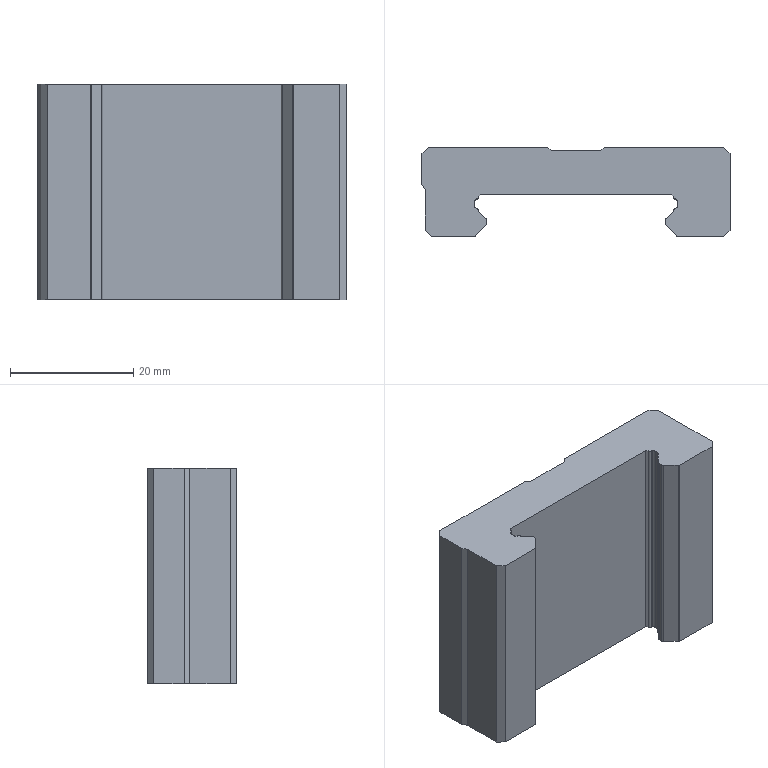Part | SolidWorks | features BaseBody 1 | 1 solid | 72 faces | box 50 x 14.5 x 35 mm | volume 17361 mm3 | plane 32 | cylinder 24 | cone 16 | commonest cylinder face diameters 1 x10 3.3 x8 0.77 x6